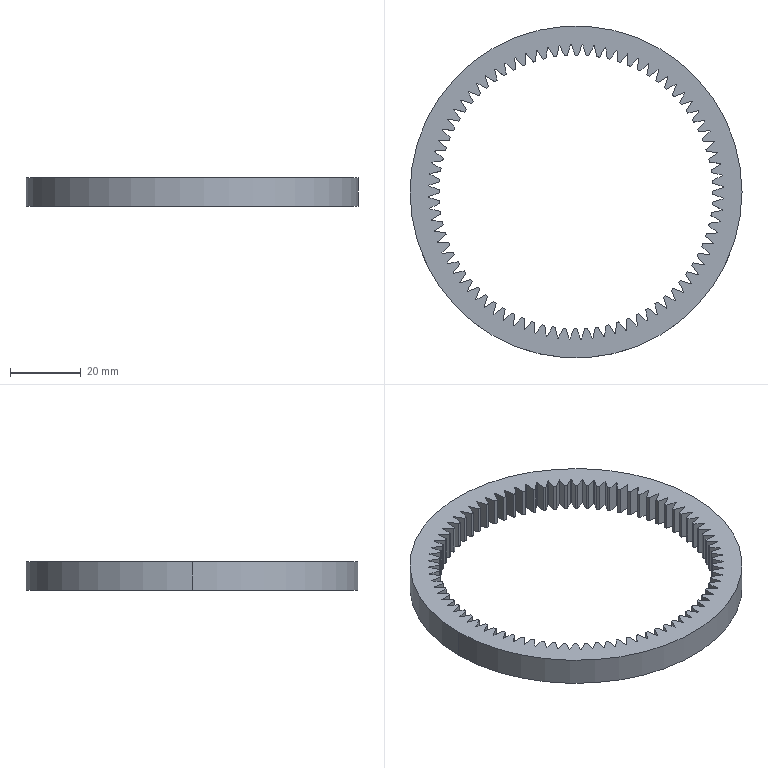Part | SolidWorks | features Cut 2, CirPattern 1, Extrusion 1, RefAxis 1 | 1 solid | 325 faces | box 94 x 94 x 8 mm | volume 15235 mm3 | cylinder 163 | spline 160 | plane 2 | commonest cylinder face diameters 77.5 x81 83.365 x80 94 x2